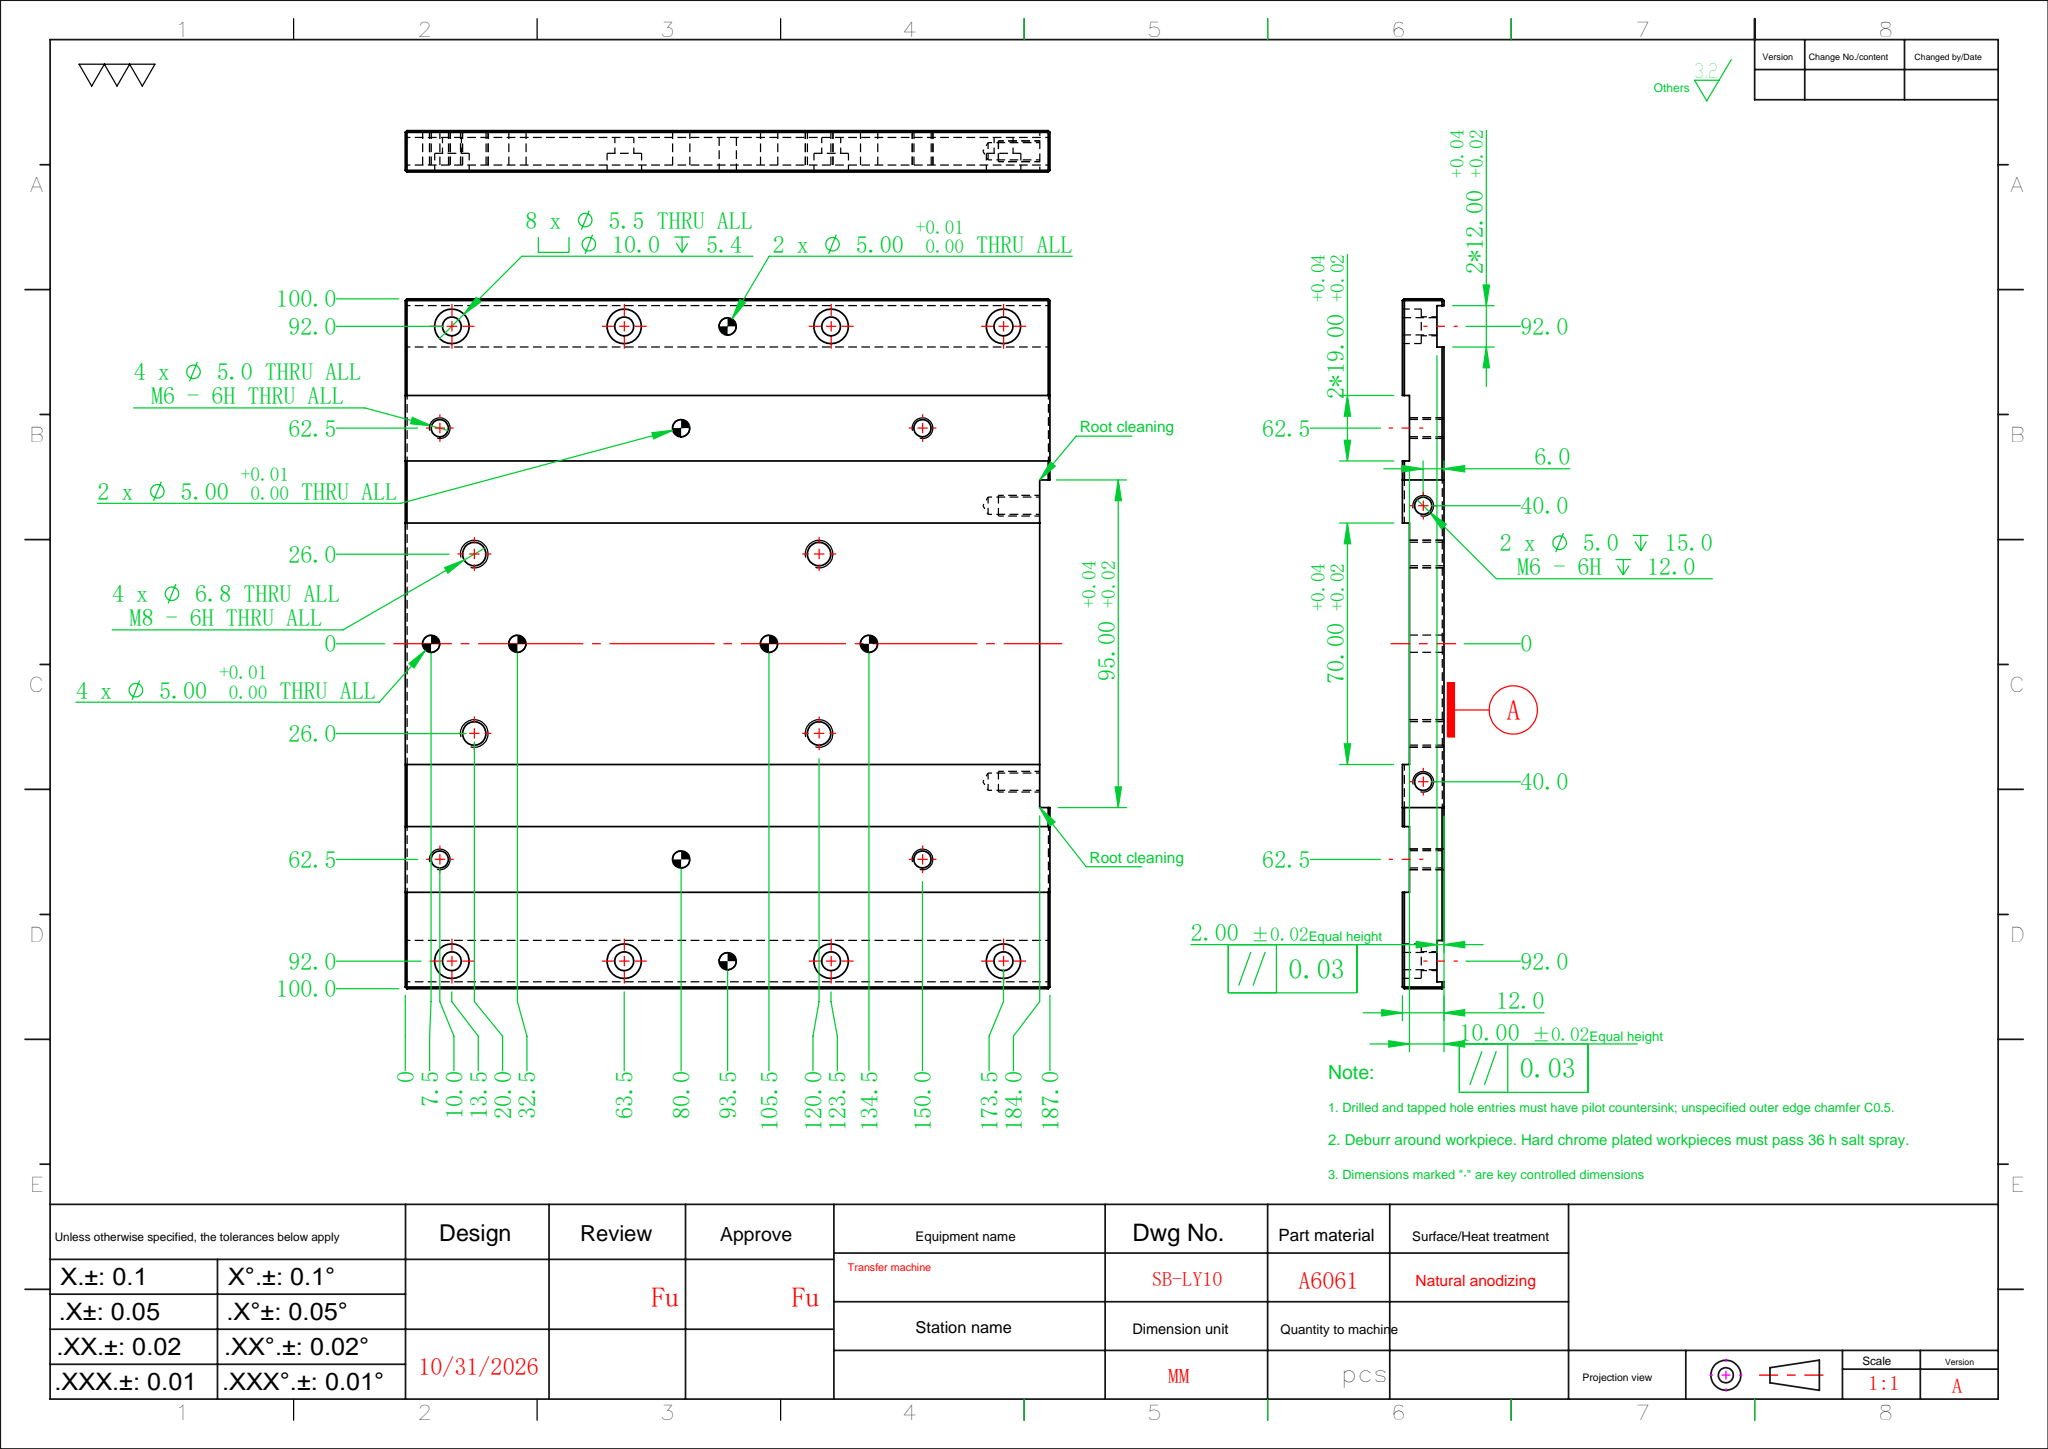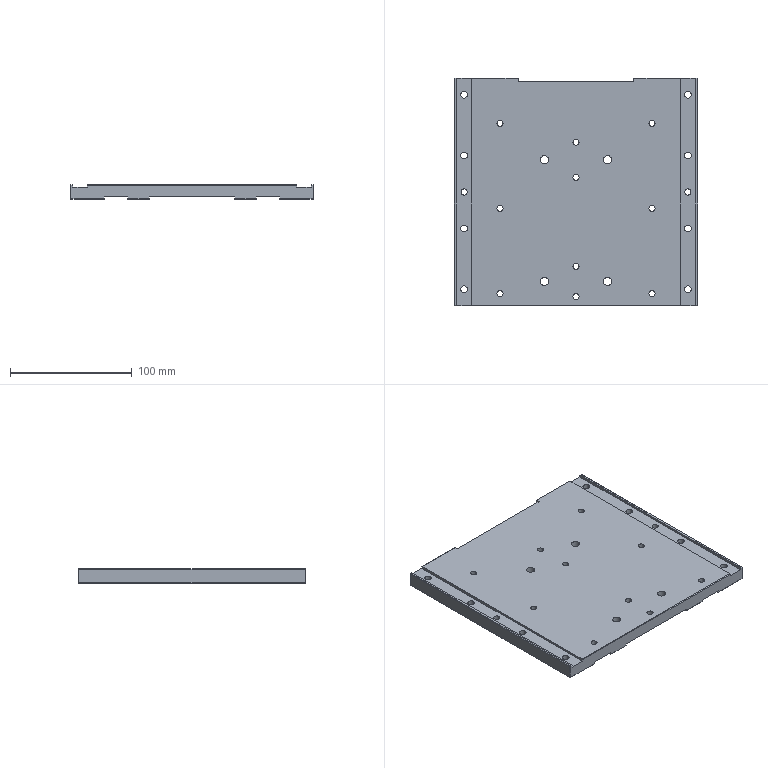Part | SolidWorks | features HoleWzd 7, Cut 4, Chamfer 1, Extrusion 1 | 1 solid | 141 faces | box 200 x 187 x 12 mm | volume 387596 mm3 | plane 69 | cylinder 68 | cone 4 | commonest cylinder face diameters 5 x28 5.5 x16 10 x16 6.8 x8